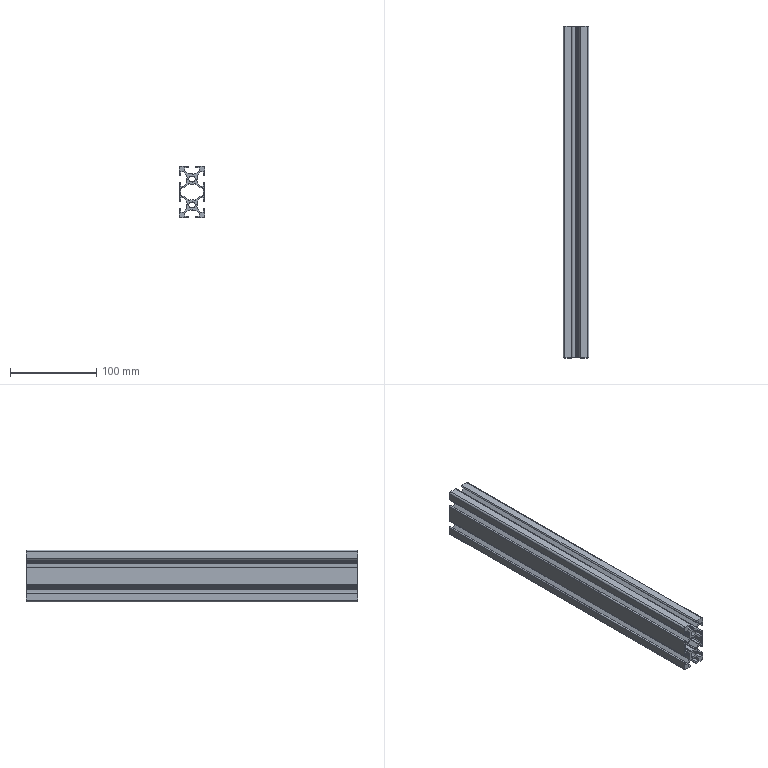Part | SolidWorks | features 3DProfileFeature 2, HoleWzd 2, WeldMemberFeat 1, WeldmentFeature 1 | 1 solid | 148 faces | box 30 x 384 x 60 mm | volume 244841 mm3 | plane 94 | cylinder 54 | commonest cylinder face diameters 2 x24 1 x13 4 x10 7 x4 12 x3